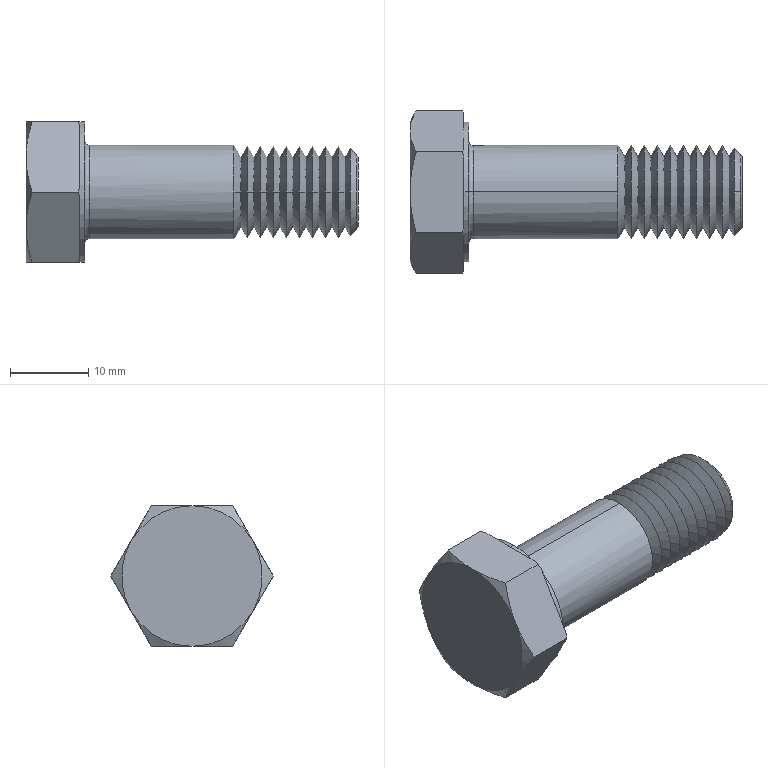Part | SolidWorks | features RevCut 4, Chamfer 1, Extrusion 1, Fillet 1, LPattern 1, Revolution 1 | 1 solid | 73 faces | box 42.5 x 20.785 x 18 mm | volume 5603 mm3 | cone 52 | plane 15 | cylinder 4 | torus 2 | commonest cylinder face diameters 12 x2 18 x2